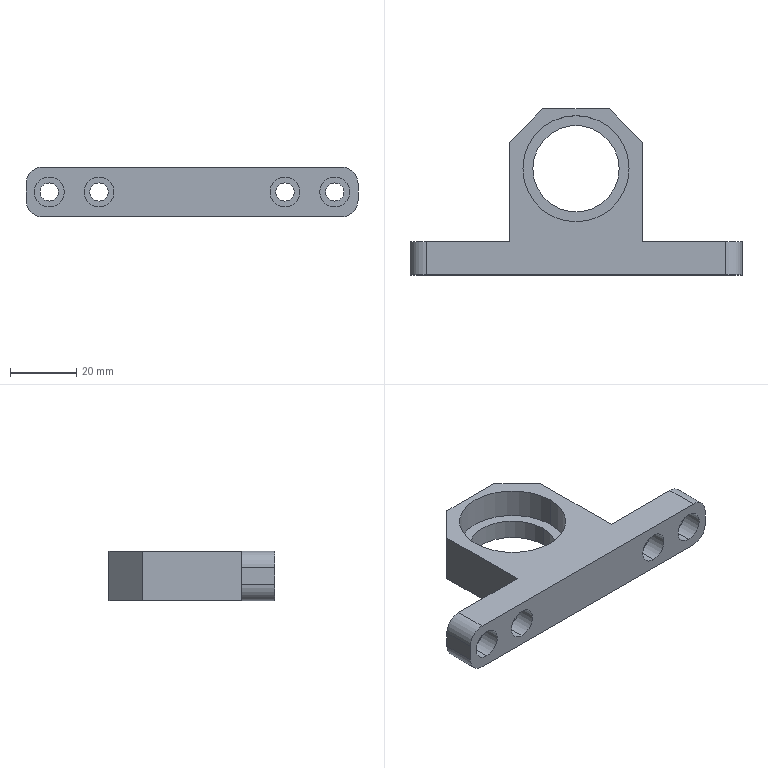Part | STEP file | B1-011 | 1 solid | 41 faces | box 100 x 50 x 15 mm | volume 24955 mm3 | cylinder 24 | plane 17 | commonest cylinder face diameters 5.5 x8 9 x8 10 x4 26 x2 32 x2